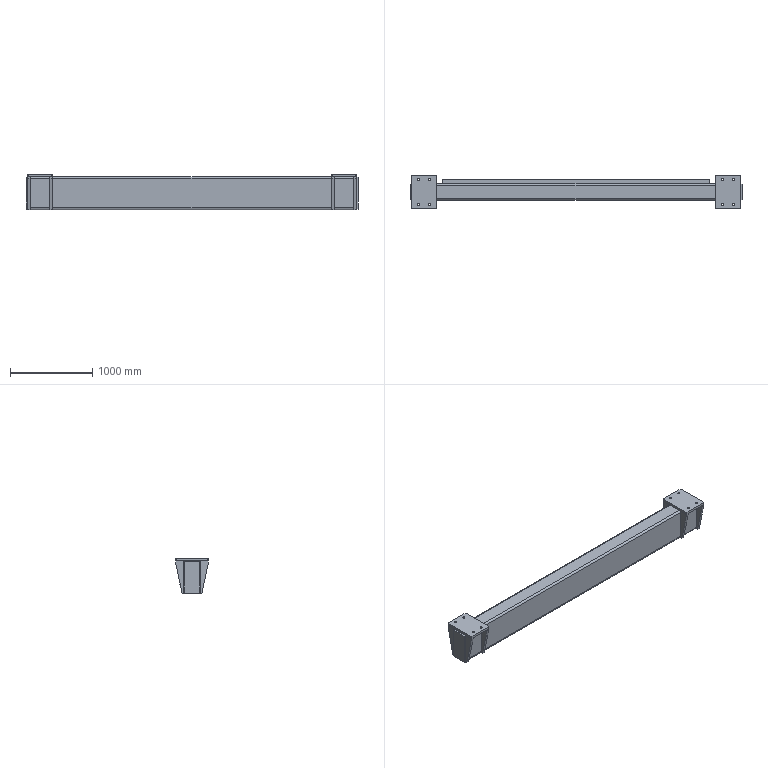Part | SolidWorks | features HoleWzd 6, ICE 4, MirrorSolid 3, Chamfer 2, EndCap 2, Cut 1, MirrorPattern 1, WeldMemberFeat 1, WeldmentFeature 1 | 16 solids | 768 faces | box 4040 x 400 x 430 mm | volume 79794691 mm3 | cone 328 | cylinder 312 | plane 128 | commonest cylinder face diameters 5 x264 26 x16 2.5 x8 6 x8 6.8 x8 24 x4